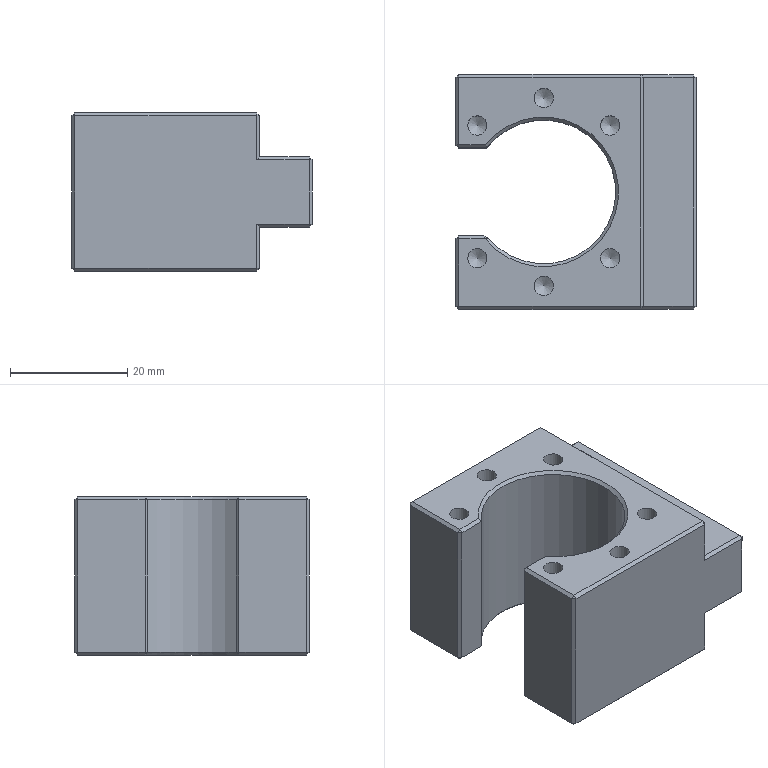CAM job | NX | 3-axis milling, drilling | part box 41 x 40 x 27 mm | stock box 46 x 45 x 30 mm
Tools:
number,name,description,diameter,corner_radius,flute_length,length,flutes
9,D10,平底铣刀-粗,10.0,0.0,35.0,75.0,2
10,D10-J,平底铣刀-精,10.0,0.0,35.0,75.0,2
1,D80R0.8飞刀,圆鼻刀-粗,80.0,0.8,50.0,75.0,2
1,D80R0.8飞刀-J,圆鼻刀-精,80.0,0.8,50.0,75.0,2
2,D6倒角刀,倒角刀,6.0,0.0,3.0,25.0,2
21,M4X0.7,丝锥,3.3,0.0,35.0,50.0,2
17,ZT12,钻头,12.0,0.0,35.0,50.0,2
13,3.3_DRILL,Twist Drill 3.3 mm,3.3,0.0,35.0,35.008,2
Operations:
program,operation,operation_type,tool,method,geometry_group,spindle_rpm,surface_speed,feed_per_tooth,feed_cut,feed_plunge,cut_length_mm,path_length_mm,cut_time_min,machine_time_min
B,FLOOR_WALL_FLY_FACE_1PASS_ROUGH_COPY,VolumeBased25DMillingOperation,D80R0.8飞刀,LAYER_ROUGH-DEPTH_K-STEP_G,W-B,2800.0,703.696,0.5357,3000.0,100.0,895.164,1904.186,0.2984,0.3993
B,FLOOR_WALL_FLY_FACE_1PASS_FINISH_COPY,VolumeBased25DMillingOperation,D80R0.8飞刀-J,SIDE_FINISH-DEPTH_K-STEP_G,W-B,4000.0,1005.28,0.125,1000.0,100.0,148.998,244.998,0.149,0.1586
B,FLOOR_WALL_LAYER_ROUGH-MID_COPY,VolumeBased25DMillingOperation,D10,LAYER_ROUGH-DEPTH_K-STEP_G,W-B,8000.0,251.32,0.25,4000.0,100.0,1599.944,1777.359,0.4,0.4177
B,FLOOR_WALL_FINISH_SIDE-MID-SELECT_FLOOR_COPY,VolumeBased25DMillingOperation,D10-J,SIDE_FINISH-DEPTH_K-STEP_G,W-B,8000.0,251.32,0.0625,1000.0,100.0,57.703,96.303,0.0577,0.0616
B,Z_LEVEL_FINISH-MID_COPY,ZLevelMilling,D10-J,SIDE_FINISH-DEPTH_K-STEP_G,W-B,8000.0,251.32,0.0625,1000.0,100.0,55.034,83.634,0.055,0.0579
B,PLANAR_DEBURR_6X45L_COPY_1,SurfaceContour,D6倒角刀,CLIMB_CHAMFER-DEPTH_0-STEP_G,W-B,6500.0,122.519,0.1154,1500.0,100.0,287.71,448.006,0.1918,0.2078
A,TOP_FACE,FaceMilling,D80R0.8飞刀,SIDE_FINISH-DEPTH_K-STEP_G,W-A,4000.0,1005.31,0.125,1000.0,100.0,135.0,171.0,0.135,0.1386
A,SPOT_DRILL-DEPTH_0.8,Operation,D6倒角刀,NONE,W-A,8000.0,150.796,0.0312,500.0,90.0,12.6,152.409,0.0252,0.0392
A,BLIND_CONE_HOLE-M4_TAP_DRILL,Operation,3.3_DRILL,NONE,W-A,3000.0,31.102,0.02,120.0,90.0,90.0,296.796,0.75,0.7707
A,THROUGH_HOLE-12.5-25,Operation,ZT12,NONE,W-A,800.0,30.159,0.125,200.0,90.0,33.605,107.21,0.168,0.1754
A,PROFILE_ROUGH_2,VolumeBased25DMillingOperation,D10,METHOD,W-A,8000.0,251.327,0.3125,5000.0,80.0,8952.704,9018.404,1.79,1.797
A,FLOOR_WALL_ROUGH_1,VolumeBased25DMillingOperation,D10,METHOD,W-A,6000.0,113.0,0.2083,3500.0,100.0,1489.5,1655.363,0.4256,0.4422
A,FLOOR_SIDE_FINISH_3,VolumeBased25DMillingOperation,D10-J,METHOD,W-A,6000.0,113.0,0.2083,1200.0,100.0,54.394,108.394,0.0453,0.0507
A,DRILL_CHAMFER_1,Operation,D6倒角刀,METHOD,W-A,8000.0,150.796,0.0312,500.0,0.0,31.2,190.657,0.0624,0.0783
A,MILL_CHAMFER_1,PlanarMilling,D6倒角刀,METHOD,W-A,8000.0,150.796,0.0625,1000.0,100.0,76.629,119.629,0.0766,0.0809
A,PLANAR_DEBURR_6X45L_COPY,SurfaceContour,D6倒角刀,CLIMB_CHAMFER-DEPTH_0-STEP_G,W-A,6500.0,122.519,0.1154,1500.0,100.0,287.712,379.761,0.1918,0.201
A,BLIND_CONE_HOLE-TAP_M4,Operation,M4X0.7,METHOD,W-A,800.0,8.294,0.0004,0.7,90.0,72.0,260.796,102.857,102.876
A,PROFILE_SEMI_FINISH_2,VolumeBased25DMillingOperation,D10-J,METHOD,W-A,8000.0,251.327,0.0625,1000.0,100.0,505.946,668.061,0.5059,0.5222